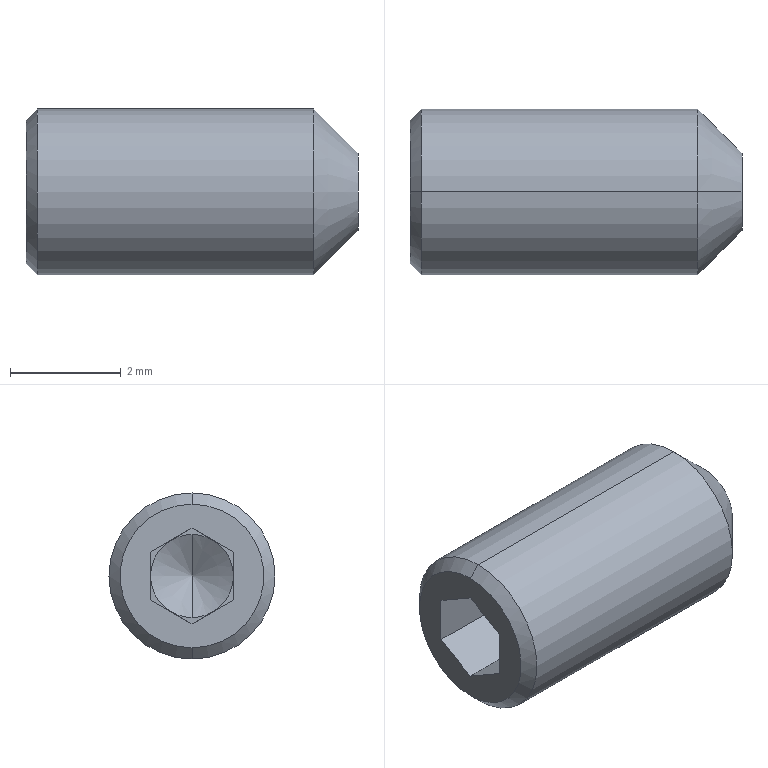Part | STEP file | 1 solid | 23 faces | box 6 x 3 x 3 mm | volume 35.386 mm3 | plane 13 | cone 8 | cylinder 2 | commonest cylinder face diameters 3 x2